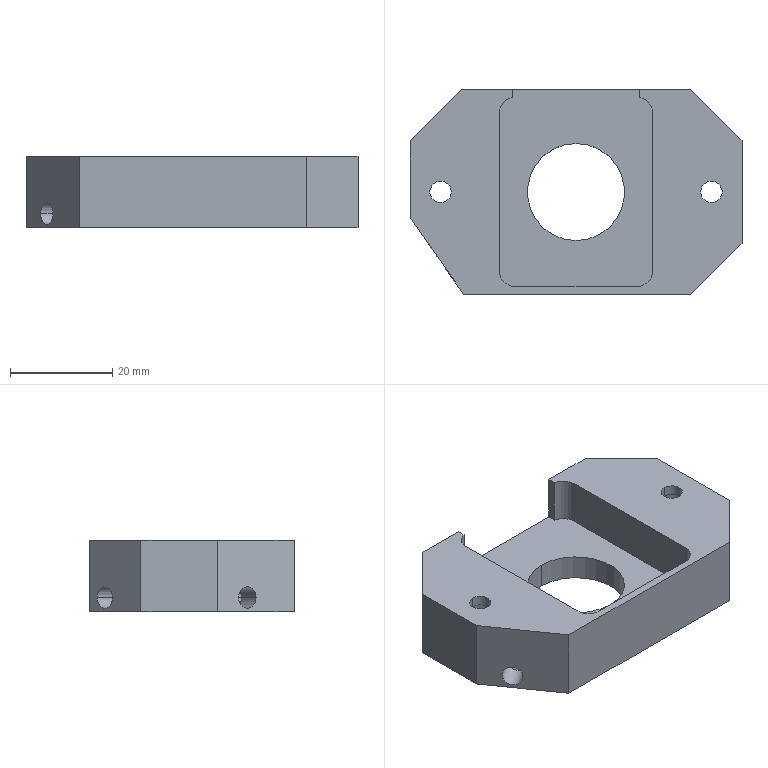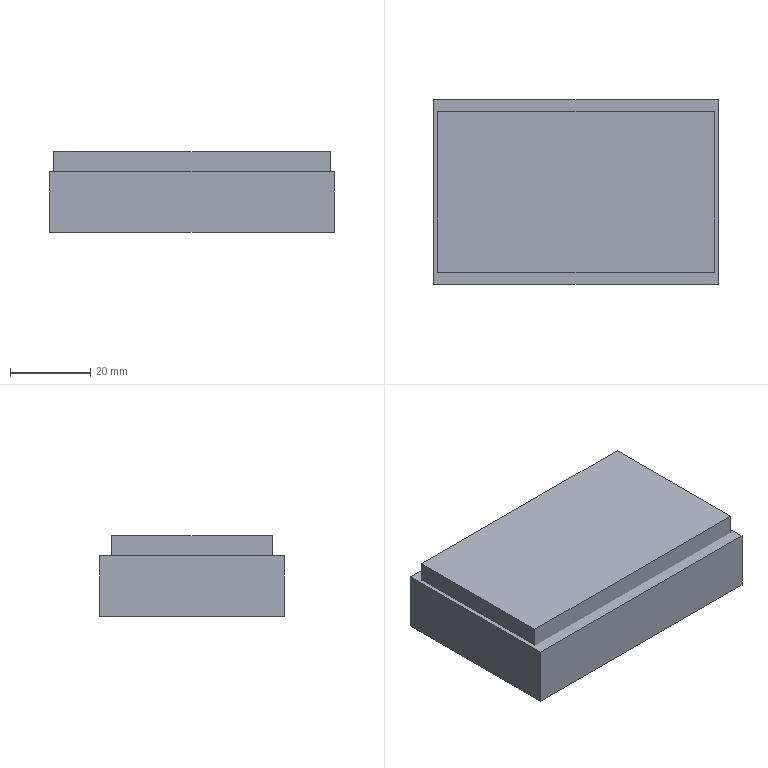CAM job | NX | 3-axis milling, drilling | part box 65 x 40 x 14 mm | stock box 71 x 46 x 20 mm
Tools:
number,name,description,diameter,corner_radius,flute_length,length,flutes
3,D50R0.8,Milling Tool-5 Parameters,50.0,0.8,50.0,75.0,2
4,D10,Milling Tool-5 Parameters,10.0,0.0,50.0,75.0,2
20,ZXZ,Milling Tool-5 Parameters,6.0,0.0,50.0,75.0,2
15,2.1ZT,Drilling Tool,2.05,0.0,35.0,50.0,2
7,1.95XYD,Thread Mill,1.95,0.0,0.45,50.0,2
12,2.0ZT,Drilling Tool,2.0,0.0,35.0,50.0,2
9,4.2ZT,Drilling Tool,4.2,0.0,35.0,50.0,2
10,3.9XYD,Thread Mill,3.9,0.0,0.8,50.0,2
6,D6,Milling Tool-5 Parameters,6.0,0.0,50.0,75.0,2
16,D6JING,Milling Tool-5 Parameters,6.0,0.0,50.0,75.0,2
14,D10JING,Milling Tool-5 Parameters,10.0,0.0,50.0,75.0,2
2,D2,Milling Tool-5 Parameters,2.0,0.0,50.0,75.0,2
1,D6A45,Milling Tool-5 Parameters,6.0,0.0,3.0,3.0,2
Operations:
program,operation,operation_type,tool,method,geometry_group,spindle_rpm,surface_speed,feed_per_tooth,feed_cut,feed_plunge,cut_length_mm,path_length_mm,cut_time_min,machine_time_min
1,FLOOR_WALL_COPY,VolumeBased25DMillingOperation,D50R0.8,METHOD,A,1500.0,296.0,0.3333,1000.0,100.0,133.0,187.0,0.133,0.1384
1,DRILLING_COPY_1,Operation,ZXZ,METHOD,A,5000.0,94.0,0.025,250.0,0.0,40.0,281.698,0.16,0.1842
1,DRILLING_COPY_1_COPY_COPY_2,Operation,2.1ZT,METHOD,A,2001.0,12.0,0.03,120.0,0.0,59.795,292.061,0.4983,0.5215
1,刀补7,ThreadMilling,1.95XYD,METHOD,A,4000.0,36.0,0.125,1000.0,100.0,377.921,1662.389,0.3779,0.5064
1,DRILLING_COPY_1_COPY_COPY_2_COPY,Operation,2.0ZT,METHOD,A,2001.0,12.0,0.03,120.0,0.0,7.601,75.202,0.0633,0.0701
1,DRILLING_COPY_1_COPY_COPY_2_COPY_1,Operation,4.2ZT,METHOD,A,2001.0,12.0,0.03,120.0,0.0,37.524,191.132,0.3127,0.3281
1,HOLE_MILLING_1,CylinderMilling,D6,METHOD,A,4000.0,75.0,0.225,1800.0,100.0,1430.902,1626.902,0.7949,0.8145
1,刀补10,ThreadMilling,3.9XYD,METHOD,A,4000.0,36.0,0.125,1000.0,100.0,76.431,813.431,0.0764,0.1501
1,ADAPTIVE_MILLING_COPY,CavityMilling,D10,METHOD,A,4000.0,125.0,0.275,2200.0,1000.0,5917.938,6001.938,2.691,2.699
1,ADAPTIVE_MILLING_COPY_COPY,CavityMilling,D10,METHOD,A,4000.0,125.0,0.275,2200.0,1000.0,1068.713,1129.713,1.022,1.028
1,ZLEVEL_PROFILE_1_COPY,ZLevelMilling,D10JING,METHOD,A,6500.0,122.0,0.0769,1000.0,100.0,221.783,307.783,0.2218,0.2304
1,ZLEVEL_PROFILE_1_COPY_COPY,ZLevelMilling,D10JING,METHOD,A,6500.0,122.0,0.0769,1000.0,100.0,34.101,102.101,0.0341,0.0409
1,ZLEVEL_PROFILE_COPY_COPY_COPY,ZLevelMilling,D2,METHOD,A,4500.0,28.0,0.1222,1100.0,1000.0,15312.772,15374.573,13.922,13.929
1,11_COPY_COPY_COPY_COPY_COPY,ZLevelMilling,D6A45,METHOD,A,7500.0,141.0,0.0667,1000.0,100.0,484.413,879.052,0.4844,0.5239
1,DRILLING_COPY_1_COPY,Operation,D6A45,METHOD,A,5000.0,94.0,0.025,250.0,0.0,26.1,224.671,0.1044,0.1243
1,刀补16,CylinderMilling,D6JING,METHOD,A,5500.0,103.0,0.0909,1000.0,100.0,96.638,292.638,0.0966,0.1162
1,DRILLING,HoleDrilling,ZXZ,METHOD,A,3500.0,65.0,0.0357,250.0,0.0,24.0,273.172,0.048,0.0729
1,DRILLING_COPY,HoleDrilling,2.0ZT,METHOD,A,2000.0,12.0,0.0125,50.0,0.0,881.814,1130.986,1.338,1.363
1,DRILLING_COPY_COPY,HoleDrilling,4.2ZT,METHOD,A,2009.0,26.0,0.0373,150.0,0.0,181.571,430.743,0.1852,0.2102
1,刀补10.,ThreadMilling,3.9XYD,METHOD,A,4000.0,49.0,0.125,1000.0,100.0,268.362,763.506,0.2684,0.3179
2,FLOOR_WALL_COPY_COPY,VolumeBased25DMillingOperation,D50R0.8,METHOD,B,1000.0,157.0,0.75,1500.0,100.0,2620.0,5957.852,1.747,2.08
2,FLOOR_WALL_COPY_COPY_1,VolumeBased25DMillingOperation,D50R0.8,METHOD,B,1500.0,296.0,0.3333,1000.0,100.0,131.0,185.0,0.131,0.1364
2,ADAPTIVE_MILLING_COPY_COPY_1,CavityMilling,D10,METHOD,B,4000.0,125.0,0.275,2200.0,1000.0,10990.719,11129.601,5.876,5.89
2,ADAPTIVE_MILLING_COPY_COPY_COPY,CavityMilling,D6,METHOD,B,4500.0,84.0,0.1667,1500.0,1000.0,503.841,1688.086,0.3409,0.4593
2,FLOOR_WALL,VolumeBased25DMillingOperation,D6JING,METHOD,B,6500.0,122.0,0.0962,1250.0,100.0,478.584,651.569,0.3829,0.4002
2,11_COPY_COPY_COPY_COPY_COPY_1,ZLevelMilling,D6A45,METHOD,B,7500.0,141.0,0.0667,1000.0,100.0,311.884,587.971,0.3119,0.3395
2,11_COPY_COPY_COPY_COPY_COPY_1_COPY,ZLevelMilling,D6A45,METHOD,B,7500.0,141.0,0.0667,1000.0,100.0,90.96,255.814,0.091,0.1074